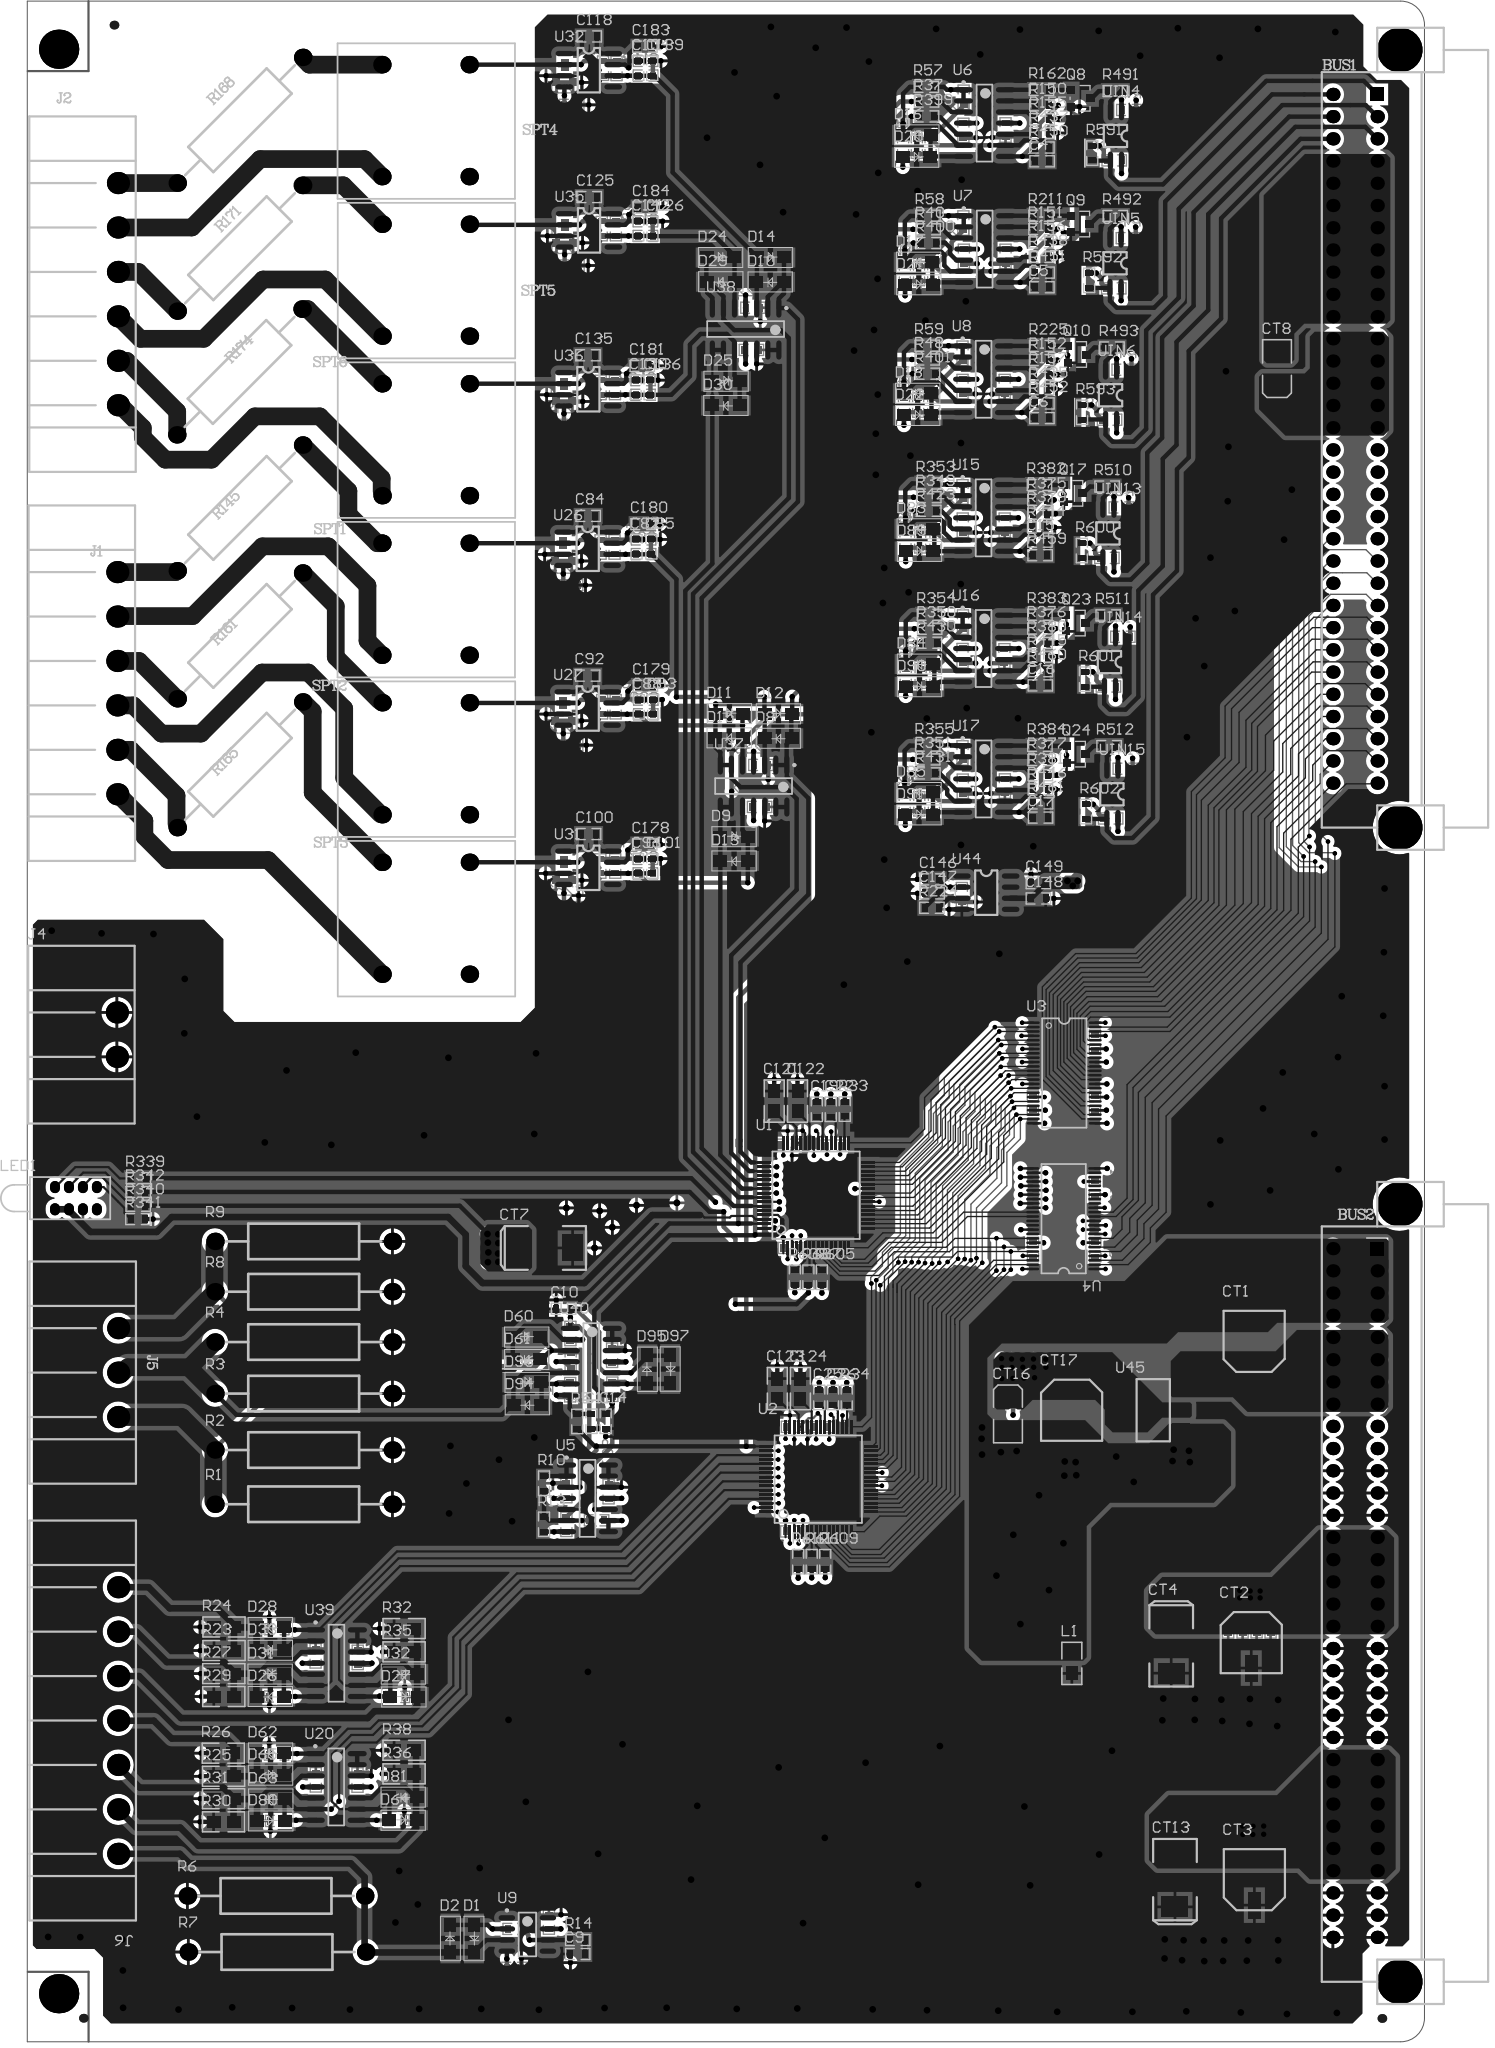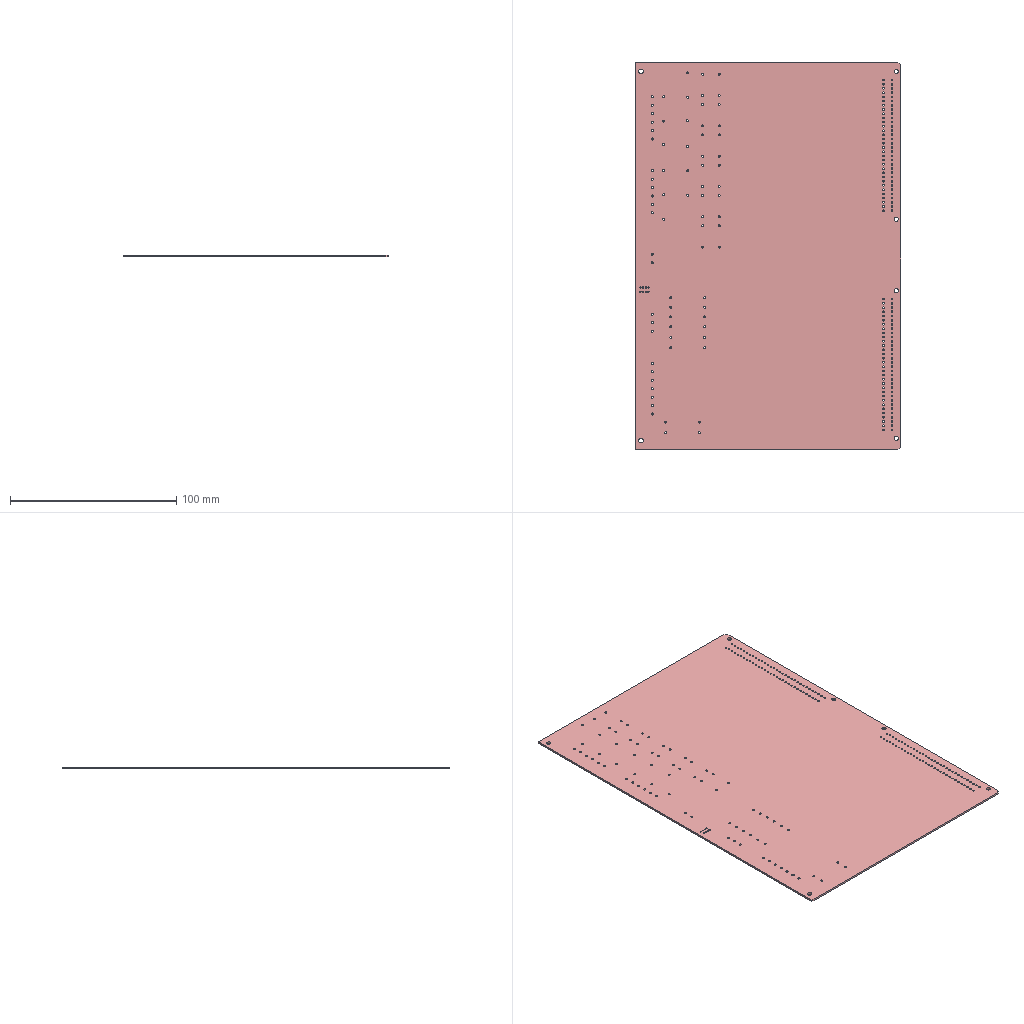Circuit board layout | Altium Designer | box 160 x 233.3 x 1.1 mm
Layer stack:
# Altium Designer layer stack of  (unit mm; dielectric type: 0 none, 1 core, 2 prepreg, 3 surface material)
index,name,kind,layer,copper_thickness_mm,dielectric_type,dielectric_thickness_mm,dielectric_material,dielectric_constant
0,TopPaste,other,,,,,,
1,TopOverlay,other,,,,,,
2,TopSolder,dielectric,,,3,0.0102,Solder Resist,3.5
3,TopLayer,copper,TopLayer,0.0356,,,,
4,Dielectric1,dielectric,,,1,0.32,FR-4,4.8
5,GND,copper,GND,0.0356,,,,
6,Dielectric2,dielectric,,,2,0.32,FR-4,4.8
7,POWER,copper,POWER,0.0356,,,,
8,Dielectric3,dielectric,,,1,0.32,FR-4,4.8
9,BottomLayer,copper,BottomLayer,0.0356,,,,
10,BottomSolder,dielectric,,,3,0.0102,Solder Resist,3.5
11,BottomOverlay,other,,,,,,
12,BottomPaste,other,,,,,,
# drill layer pairs: low layer,high layer
drill_pair,TopLayer,BottomLayer
Part placement:
Designator,Comment,Layer,Footprint,Center-X(mm),Center-Y(mm),Rotation
C253,0.1uF,BottomLayer,0603,62.306,129.743,180
C252,0.1uF,BottomLayer,0603,62.23,166.548,360
C251,0.1uF,BottomLayer,0603,62.382,203.098,180
C224,0.1uF,BottomLayer,0603,83.109,198.272,360
C194,0.1uF,BottomLayer,0603,37.846,43.967,270
R28,0,BottomLayer,0603,61.747,59.182,270
R12,10k_1%,BottomLayer,0603,65.202,59.639,360
C1,0.1uF,BottomLayer,0603,115.189,90.602,90
C2,0.1uF,BottomLayer,0603,122.326,90.602,270
C7,0.1uF,BottomLayer,0603,122.276,107.315,90
C8,0.1uF,BottomLayer,0603,115.164,107.34,270
R11,4.7k,BottomLayer,0603,55.88,12.929,180
C12,30p,BottomLayer,0603,28.575,47.193,360
C13,30p,BottomLayer,0603,28.55,32.868,360
C20,30p,BottomLayer,0603,28.575,39.497,360
C21,30p,BottomLayer,0603,28.677,25.273,360
C23,30p,BottomLayer,0603,42.393,39.446,180
C27,30p,BottomLayer,0603,42.342,25.349,180
C3,0.1uF,BottomLayer,0603,112.903,73.863,270
C18,1uF,BottomLayer,0603,92.329,102.489,360
C24,1uF,BottomLayer,0603,87.757,70.333,360
C83,1000p,BottomLayer,0603,70.587,170.104,360
C89,1000p,BottomLayer,0603,70.841,151.79,360
C97,1000p,BottomLayer,0603,70.79,133.604,360
C113,1000p,BottomLayer,0603,70.815,224.815,360
C119,0.1uF,BottomLayer,0603,87.046,102.591,360
C120,0.1uF,BottomLayer,0603,90.907,70.282,180
C128,0.1uF,BottomLayer,0603,87.427,90.78,360
C129,0.1uF,BottomLayer,0603,87.681,58.369,360
C132,1000p,BottomLayer,0603,70.536,188.316,360
C143,1000p,BottomLayer,0603,70.79,206.477,360
C156,0.1uF,BottomLayer,0603,124.485,215.113,360
C157,0.1uF,BottomLayer,0603,124.435,200.482,180
C158,0.1uF,BottomLayer,0603,123.952,185.471,180
C159,0.1uF,BottomLayer,0603,123.647,169.672,360
C163,0.1uF,BottomLayer,0603,123.825,154.965,180
C164,0.1uF,BottomLayer,0603,124.079,139.878,180
C165,0.1uF,BottomLayer,0603,122.276,114.3,270
C171,0.1uF,BottomLayer,0603,122.25,97.561,90
C173,0.1uF,BottomLayer,0603,137.541,47.574,90
C174,0.1uF,BottomLayer,0603,139.192,47.574,270
C175,0.1uF,BottomLayer,0603,140.792,47.6,270
C176,0.1uF,BottomLayer,0603,142.392,47.574,90
C177,0.1uF,BottomLayer,0603,61.747,63.043,90
C182,0.1uF,BottomLayer,0603,55.855,89.179,180
C192,0.1uF,BottomLayer,0603,37.821,29.947,270
C193,0.1uF,BottomLayer,0603,112.039,204.14,270
C195,0.1uF,BottomLayer,0603,55.753,8.484,360
C196,0.1uF,BottomLayer,0603,66.573,62.916,90
C197,0.1uF,BottomLayer,0603,66.98,78.511,270
C204,0.1uF,BottomLayer,0603,142.215,21.615,90
C205,0.1uF,BottomLayer,0603,140.589,21.59,90
C206,0.1uF,BottomLayer,0603,138.963,21.59,270
C215,0.1uF,BottomLayer,0603,107.213,218.542,270
C216,0.1uF,BottomLayer,0603,107.036,131.166,90
C217,0.1uF,BottomLayer,0603,107.112,158.496,90
C218,0.1uF,BottomLayer,0603,107.137,173.406,270
C219,0.1uF,BottomLayer,0603,107.264,204.14,90
C220,0.1uF,BottomLayer,0603,59.741,13.716,270
C230,0.1uF,BottomLayer,0603,33.045,29.972,270
C231,0.1uF,BottomLayer,0603,107.137,143.561,270
C232,0.1uF,BottomLayer,0603,107.112,189.255,270
C233,0.1uF,BottomLayer,0603,84.023,145.999,180
C234,0.1uF,BottomLayer,0603,62.23,77.927,90
C235,0.1uF,BottomLayer,0603,33.02,44.145,270
C238,0.1uF,BottomLayer,0603,111.912,158.471,90
C239,0.1uF,BottomLayer,0603,111.938,189.255,270
C240,0.1uF,BottomLayer,0603,82.931,193.446,360
C249,0.1uF,BottomLayer,0603,62.306,184.887,360
C254,0.1uF,BottomLayer,0603,62.23,148.26,360
C255,0.1uF,BottomLayer,0603,111.963,143.586,270
C256,0.1uF,BottomLayer,0603,111.938,173.406,90
C257,0.1uF,BottomLayer,0603,112.039,218.592,90
C261,0.1uF,BottomLayer,0603,62.357,221.463,180
C262,0.1uF,BottomLayer,0603,83.871,141.199,360
D42,BAV99W,BottomLayer,SOT23R,61.404,170.332,180
D44,BAV99W,BottomLayer,SOT23R,61.404,152.07,180
D46,BAV99W,BottomLayer,SOT23R,61.481,133.833,180
D48,BAV99W,BottomLayer,SOT23R,61.557,225.044,180
D51,BAV99W,BottomLayer,SOT23R,61.557,206.705,180
D53,BAV99W,BottomLayer,SOT23R,61.481,188.57,180
R67,10k,BottomLayer,0603,100.305,216.738,90
R70,10k,BottomLayer,0603,100.508,202.184,90
R71,10k,BottomLayer,0603,100.406,187.147,90
R76,10k,BottomLayer,0603,107.239,222.326,90
R85,4.7k,BottomLayer,0603,67.005,74.625,90
R86,10k,BottomLayer,0603,107.213,207.95,90
R87,10k,BottomLayer,0603,107.112,193.065,90
R93,4.7k,BottomLayer,0603,62.179,74.574,90
R97,4.7k,BottomLayer,0603,62.205,81.001,270
R100,10k,BottomLayer,0603,103.454,216.738,270
R105,5.1k_1%,BottomLayer,0603,65.659,189.154,90
R106,5.1k_1%,BottomLayer,0603,67.31,189.154,90
R108,10k,BottomLayer,0603,103.759,202.209,270
R110,5.1k_1%,BottomLayer,0603,67.412,207.315,90
R111,5.1k_1%,BottomLayer,0603,65.786,207.315,90
R113,5.1k,BottomLayer,0603,70.79,208.153,180
R117,10k,BottomLayer,0603,103.759,187.147,270
R118,5.1k,BottomLayer,0603,70.815,226.492,180
R119,5.1k_1%,BottomLayer,0603,67.488,225.628,90
R120,5.1k_1%,BottomLayer,0603,65.938,225.654,90
R124,5.1k,BottomLayer,0603,70.79,135.255,180
R125,5.1k_1%,BottomLayer,0603,67.335,134.442,90
R126,5.1k_1%,BottomLayer,0603,65.634,134.442,90
R130,5.1k,BottomLayer,0603,70.841,153.467,180
R131,5.1k_1%,BottomLayer,0603,65.837,152.654,90
R132,10k,BottomLayer,0603,101.879,216.738,270
R133,5.1k_1%,BottomLayer,0603,67.386,152.654,90
R137,5.1k,BottomLayer,0603,70.587,171.78,180
R138,5.1k_1%,BottomLayer,0603,65.659,170.917,90
R139,5.1k_1%,BottomLayer,0603,67.259,170.917,90
R146,10k,BottomLayer,0603,102.133,202.184,270
R147,10k,BottomLayer,0603,102.032,187.147,270
R357,10k,BottomLayer,0603,100.584,171.679,90
R358,10k,BottomLayer,0603,100.609,156.185,90
R359,10k,BottomLayer,0603,100.482,141.554,90
R360,10k,BottomLayer,0603,107.112,177.216,90
R361,10k,BottomLayer,0603,107.163,162.331,90
R362,10k,BottomLayer,0603,107.112,147.371,90
R364,10k,BottomLayer,0603,102.26,171.628,270
R365,10k,BottomLayer,0603,102.311,156.159,270
R366,10k,BottomLayer,0603,103.835,141.554,270
R372,10k,BottomLayer,0603,104.013,171.628,270
R373,10k,BottomLayer,0603,104.013,156.185,270
R374,10k,BottomLayer,0603,102.159,141.554,270
R414,5.1k,BottomLayer,0603,70.536,189.992,180
R486,2k,BottomLayer,0603,126.162,220.878,180
R487,2k,BottomLayer,0603,126.111,206.223,180
R488,2k,BottomLayer,0603,125.628,191.186,180
R503,2k,BottomLayer,0603,125.298,175.438,180
R506,2k,BottomLayer,0603,125.476,160.655,180
R507,2k,BottomLayer,0603,125.755,145.567,180
R342,3.3k,TopLayer,0603,12.7,97.18,360
R38,2k,TopLayer,0805,43.155,33.35,180
R36,2k,TopLayer,0805,43.155,30.658,180
R35,2k,TopLayer,0805,43.155,44.602,180
R32,2k,TopLayer,0805,43.155,47.269,180
R31,2k,TopLayer,0805,22.479,27.813,180
R30,2k,TopLayer,0805,22.479,25.171,180
R29,2k,TopLayer,0805,22.504,39.497,180
R27,2k,TopLayer,0805,22.504,42.113,180
R26,2k,TopLayer,0805,22.454,33.02,180
R25,2k,TopLayer,0805,22.479,30.378,180
R24,2k,TopLayer,0805,22.53,47.447,180
R23,2k,TopLayer,0805,22.53,44.755,180
U5,TL064I,TopLayer,TL064D_SOIC-14,64.16,62.154,0
R13,10k_1%,TopLayer,0603,59.182,59.182,90
R10,10k_1%,TopLayer,0603,59.182,63.881,90
R5,0,TopLayer,0603,62.992,70.942,90
J5,Header3,TopLayer,EDGCON_3p_5.08mm_ear,10.414,76.53,270
SPT6,SPT204A,TopLayer,SPT204A,45.64,183.184,360
SPT5,SPT204A,TopLayer,SPT204A,45.64,201.421,360
SPT4,SPT204A,TopLayer,SPT204A,45.615,219.658,360
SPT3,SPT204A,TopLayer,SPT204A,45.64,128.472,360
SPT2,SPT204A,TopLayer,SPT204A,45.64,146.71,360
SPT1,SPT204A,TopLayer,SPT204A,45.615,164.947,360
R174,50kO_2W_1%,TopLayer,AXIAL0.8,24.309,190.925,225
R171,50kO_2W_1%,TopLayer,AXIAL0.8,24.36,205.073,225
R168,50kO_2W_1%,TopLayer,AXIAL0.8,24.36,219.703,225
R165,50kO_2W_1%,TopLayer,AXIAL0.8,24.36,146.018,225
R161,50kO_2W_1%,TopLayer,AXIAL0.8,24.36,160.75,225
R145,50kO_2W_1%,TopLayer,AXIAL0.8,24.36,175.38,225
BUS2,CON64,TopLayer,BUS64W-A,153.34,51.333,270
BUS1,CON64,TopLayer,BUS64W-A,153.34,183.286,270
J1,CON6,TopLayer,EDGCon_6P_5.08mm_ear,10.312,155.346,270
J2,CON6,TopLayer,EDGCon_6P_5.08mm_ear,10.389,199.822,270
U3,SN74LVCH16T245_TSSOP48,TopLayer,SN74LVC16245_TSSOP48,118.764,110.779,0
U4,SN74LVCH16T245_TSSOP48,TopLayer,SN74LVC16245_TSSOP48,118.7,94.123,180
D1,1N4148,TopLayer,1N4148-A,51.156,11.836,270
D2,1N4148,TopLayer,1N4148-A,48.463,11.836,90
R6,2W_1%,TopLayer,AXIAL0.8,28.49,16.701,360
R7,2W_1%,TopLayer,AXIAL0.8,28.6,10.287,360
U9,TL061D,TopLayer,TL061_SOIC8,57.277,12.294,0
C9,0.1uF,TopLayer,0603,63.043,10.058,0
R14,10k,TopLayer,0603,63.043,11.659,180
LED1,LEDGroup_4,TopLayer,LEDGroup_4,5.575,96.469,360
J4,Header2,TopLayer,EDGCON_2p_5.08mm_ear,10.262,115.164,270
J6,Header7,TopLayer,EDGCon_7P_5.08mm_ear,10.414,36.754,270
C10,30p,TopLayer,0603,61.417,83.82,360
C11,30p,TopLayer,0603,64.618,70.968,90
C14,30p,TopLayer,0603,66.243,70.968,90
C4,0.1uF,TopLayer,0603,116.23,215.011,360
C5,0.1uF,TopLayer,0603,116.205,200.609,360
C6,0.1uF,TopLayer,0603,116.205,185.649,0
C15,0.1uF,TopLayer,0603,115.976,171.526,360
C16,0.1uF,TopLayer,0603,116.027,155.092,360
C17,0.1uF,TopLayer,0603,116.053,139.979,360
C19,1uF,TopLayer,0603,90.424,106.629,270
C22,1uF,TopLayer,0603,92.024,106.629,270
C25,1uF,TopLayer,0603,90.703,73.685,270
C26,1uF,TopLayer,0603,92.278,73.685,270
C82,680p,TopLayer,0603,69.774,170.942,90
C84,30p,TopLayer,0603,64.237,174.473,180
C85,30p,TopLayer,0603,71.476,170.942,270
C88,680p,TopLayer,0603,70.028,152.629,90
C92,30p,TopLayer,0603,64.186,156.21,180
C93,30p,TopLayer,0603,71.679,152.629,270
C96,680p,TopLayer,0603,69.952,134.442,90
C100,30p,TopLayer,0603,64.287,138.1,180
C101,30p,TopLayer,0603,71.577,134.442,270
C104,680p,TopLayer,0603,69.977,225.654,90
C118,30p,TopLayer,0603,64.364,229.286,180
C121,10u,TopLayer,0805,85.547,107.569,270
C122,10u,TopLayer,0805,88.214,107.569,270
C123,10u,TopLayer,0805,85.903,74.701,270
C124,10u,TopLayer,0805,88.544,74.701,270
C125,30p,TopLayer,0603,64.364,210.922,180
C126,30p,TopLayer,0603,71.603,207.315,270
C130,680p,TopLayer,0603,69.672,189.179,90
C135,30p,TopLayer,0603,64.211,192.837,180
C136,30p,TopLayer,0603,71.272,189.154,270
C139,30p,TopLayer,0603,71.577,225.654,270
C142,680p,TopLayer,0603,69.977,207.315,90
C146,1uF,TopLayer,0603,103.632,132.918,180
C147,0.1uF,TopLayer,0603,103.632,131.318,180
C148,1uF,TopLayer,0603,115.799,130.734,360
C149,0.1uF,TopLayer,0603,115.799,132.486,360
C178,0.1uF,TopLayer,0603,70.714,136.906,180
C179,0.1uF,TopLayer,0603,70.79,155.042,180
C180,0.1uF,TopLayer,0603,70.536,173.533,360
C181,0.1uF,TopLayer,0603,70.434,191.618,360
C183,0.1uF,TopLayer,0603,70.739,228.117,180
C184,0.1uF,TopLayer,0603,70.764,209.728,360
CT1,100uF/16V,TopLayer,L470UF,140.513,80.099,180
CT2,100uF/35V,TopLayer,L470UF,140.183,45.657,0
CT3,100uF/35V,TopLayer,L470UF,140.538,18.555,180
CT8,22u/16V,TopLayer,3528_CASE-B,143.129,191.376,90
CT17,100uF/16V,TopLayer,L470UF,119.609,72.225,360
D8,1N4148,TopLayer,1N4148-A,86.03,149.047,180
D9,1N4148,TopLayer,1N4148-A,80.95,137.795,360
D10,1N4148,TopLayer,1N4148-A,85.09,201.219,180
D11,1N4148,TopLayer,1N4148-A,80.416,151.867,360
D12,1N4148,TopLayer,1N4148-A,86.03,151.841,360
D13,1N4148,TopLayer,1N4148-A,80.95,135.026,180
D14,1N4148,TopLayer,1N4148-A,85.115,204.013,360
D15,1N4148,TopLayer,1N4148-A,80.391,149.098,180
D16,1N4148,TopLayer,1N4148-A,101.879,218.034,180
D17,1N4148,TopLayer,1N4148-A,102.083,203.479,180
D18,1N4148,TopLayer,1N4148-A,101.981,188.493,180
D20,1N4148,TopLayer,1N4148-A,101.854,215.468,360
D21,1N4148,TopLayer,1N4148-A,102.108,200.889,360
D22,1N4148,TopLayer,1N4148-A,101.981,185.953,360
D24,1N4148,TopLayer,1N4148-A,79.4,204.013,360
D25,1N4148,TopLayer,1N4148-A,80.035,189.865,360
D26,1N4148,TopLayer,1N4148-A,27.838,39.497,180
D27,1N4148,TopLayer,1N4148-A,43.129,39.446,360
D28,1N4148,TopLayer,1N4148-A,27.838,47.396,180
D29,1N4148,TopLayer,1N4148-A,79.426,201.244,180
D30,1N4148,TopLayer,1N4148-A,80.01,187.096,180
D31,1N4148,TopLayer,1N4148-A,27.813,42.062,360
D32,1N4148,TopLayer,1N4148-A,43.078,42.062,180
D33,1N4148,TopLayer,1N4148-A,27.838,44.78,360
D60,1N4148,TopLayer,1N4148-A,57.201,80.594,360
D61,1N4148,TopLayer,1N4148-A,57.201,78.029,180
D62,1N4148,TopLayer,1N4148-A,27.864,33.045,180
D63,1N4148,TopLayer,1N4148-A,27.889,27.788,180
D64,1N4148,TopLayer,1N4148-A,43.053,25.349,360
D65,1N4148,TopLayer,1N4148-A,27.864,30.505,360
D80,1N4148,TopLayer,1N4148-A,27.889,25.273,360
D81,1N4148,TopLayer,1N4148-A,43.053,27.991,180
D83,1N4148,TopLayer,1N4148-A,102.159,172.999,180
D84,1N4148,TopLayer,1N4148-A,102.184,157.531,180
D85,1N4148,TopLayer,1N4148-A,102.133,142.85,180
D89,1N4148,TopLayer,1N4148-A,102.184,170.409,360
D90,1N4148,TopLayer,1N4148-A,102.184,154.94,360
D91,1N4148,TopLayer,1N4148-A,102.133,140.284,360
D94,1N4148,TopLayer,1N4148-A,57.277,72.847,180
D95,1N4148,TopLayer,1N4148-A,71.018,76.911,90
D96,1N4148,TopLayer,1N4148-A,57.252,75.413,360
D97,1N4148,TopLayer,1N4148-A,73.635,76.937,270
L1,1uH,TopLayer,0805,119.634,43.282,270
Q8,2N2222,TopLayer,SOT23-3,120.637,222.212,270
Q9,2N2222,TopLayer,SOT23-3,120.587,207.835,270
Q10,2N2222,TopLayer,SOT23-3,120.231,192.926,270
Q17,2N2222,TopLayer,SOT23-3,119.799,177.051,270
Q23,2N2222,TopLayer,SOT23-3,120.079,162.217,270
Q24,2N2222,TopLayer,SOT23-3,120.104,147.231,270
R1,100O_2W_1%,TopLayer,AXIAL0.8,31.657,61.48,180
R2,100O_2W_1%,TopLayer,AXIAL0.8,31.657,67.678,180
R3,100O_2W_1%,TopLayer,AXIAL0.8,31.657,74.129,180
R4,100O_2W_1%,TopLayer,AXIAL0.8,31.657,80.022,180
R8,100O_2W_1%,TopLayer,AXIAL0.8,31.657,85.776,180
R9,100O_2W_1%,TopLayer,AXIAL0.8,31.657,91.528,180
R33,10k,TopLayer,0603,93.624,106.655,90
R34,10k,TopLayer,0603,93.853,73.685,90
R37,10k,TopLayer,0603,102.997,221.844,180
R40,10k,TopLayer,0603,103.175,207.239,180
R48,10k,TopLayer,0603,103.073,192.354,180
R57,10k,TopLayer,0603,102.972,223.52,360
R58,10k,TopLayer,0603,103.149,208.788,360
R59,10k,TopLayer,0603,103.073,193.929,360
R150,10k,TopLayer,0603,116.205,221.412,360
R151,10k,TopLayer,0603,116.103,207.264,360
R152,10k,TopLayer,0603,116.18,192.278,360
R155,10k,TopLayer,0603,116.23,219.837,360
R156,10k,TopLayer,0603,116.103,205.74,360
R157,10k,TopLayer,0603,116.18,190.627,360
R162,10k,TopLayer,0603,116.154,223.164,180
R211,10k,TopLayer,0603,116.103,208.788,180
R224,0,TopLayer,0603,103.607,129.667,180
R225,10k,TopLayer,0603,116.18,193.904,180
R339,3.3k,TopLayer,0603,12.725,98.755,360
R340,10k,TopLayer,0603,12.7,95.606,360
R341,10k,TopLayer,0603,12.675,94.082,360
R349,10k,TopLayer,0603,103.251,176.606,180
R350,10k,TopLayer,0603,103.353,161.569,180
R351,10k,TopLayer,0603,103.124,146.634,180
R353,10k,TopLayer,0603,103.251,178.181,360
R354,10k,TopLayer,0603,103.327,163.17,360
R355,10k,TopLayer,0603,103.124,148.209,360
R375,10k,TopLayer,0603,115.976,176.301,360
R376,10k,TopLayer,0603,115.976,161.595,360
R377,10k,TopLayer,0603,116.002,146.558,360
R379,10k,TopLayer,0603,115.976,174.727,360
R380,10k,TopLayer,0603,116.002,159.944,360
R381,10k,TopLayer,0603,116.027,144.831,360
R382,10k,TopLayer,0603,115.926,178.003,180
R383,10k,TopLayer,0603,115.976,163.17,180
R384,10k,TopLayer,0603,115.976,148.184,180
R399,5.1k,TopLayer,0603,102.997,220.142,180
R400,5.1k,TopLayer,0603,103.2,205.664,180
R401,5.1k,TopLayer,0603,103.099,190.729,180
R423,5.1k,TopLayer,0603,103.251,175.057,180
R430,5.1k,TopLayer,0603,103.327,159.969,180
R431,5.1k,TopLayer,0603,103.149,145.034,180
R435,2.4k,TopLayer,0603,116.18,188.951,360
R437,2.4k,TopLayer,0603,116.205,218.237,360
R438,2.4k,TopLayer,0603,116.154,204.089,360
R444,2.4k,TopLayer,0603,115.951,173.152,360
R445,2.4k,TopLayer,0603,116.027,158.369,360
R446,2.4k,TopLayer,0603,116.027,143.205,360
R450,5.6k,TopLayer,0603,116.205,216.586,360
R451,5.6k,TopLayer,0603,116.23,202.286,360
R452,5.6k,TopLayer,0603,116.205,187.325,360
R459,5.6k,TopLayer,0603,116.002,169.977,360
R460,5.6k,TopLayer,0603,116.027,156.718,360
R461,5.6k,TopLayer,0603,116.053,141.605,360
R491,2k,TopLayer,0603,124.612,223.037,180
R492,2k,TopLayer,0603,124.612,208.763,180
R493,2k,TopLayer,0603,124.231,193.726,180
R510,2k,TopLayer,0603,123.673,177.825,180
R511,2k,TopLayer,0603,123.8,163.093,180
R512,2k,TopLayer,0603,123.901,148.158,180
R591,10k,TopLayer,0603,121.971,215.951,270
R592,10k,TopLayer,0603,121.615,201.397,270
R593,10k,TopLayer,0603,120.802,186.309,270
R600,10k,TopLayer,0603,120.777,170.51,270
R601,10k,TopLayer,0603,121.133,155.804,270
R602,10k,TopLayer,0603,121.26,140.665,270
R605,4.7k,TopLayer,0603,91.008,87.427,270
R607,4.7k,TopLayer,0603,89.459,87.427,270
R608,4.7k,TopLayer,0603,87.909,87.427,270
R609,4.7k,TopLayer,0603,91.389,54.915,270
R611,4.7k,TopLayer,0603,89.84,54.915,270
R612,4.7k,TopLayer,0603,88.29,54.915,270
U26,OP07CS,TopLayer,SO-8,64.186,170.713,0
U27,OP07CS,TopLayer,SO-8,64.186,152.451,0
U31,OP07CS,TopLayer,SO-8,64.262,134.239,0
U32,OP07CS,TopLayer,SO-8,64.313,225.425,0
U35,OP07CS,TopLayer,SO-8,64.338,207.112,0
U36,OP07CS,TopLayer,SO-8,64.262,188.951,0
U44,REF195,TopLayer,SO-8,109.83,131.394,360
U45,AS1117-3.3V,TopLayer,SOT223,128.956,72.225,90
CT4,22u/35V,TopLayer,7343_CASE-D,131.013,45.288,90
CT7,22u/35V,TopLayer,7343_CASE-D,59.334,90.78,180
CT13,22u/35V,TopLayer,7343_CASE-D,131.445,18.567,270
CT16,22u/16V,TopLayer,3528_CASE-B,112.319,71.742,270
U1,AD7606,TopLayer,AD7606_LQFP64,90.339,96.805,90
U2,AD7606,TopLayer,AD7606_LQFP64,90.593,64.344,90
U6,TL064I,TopLayer,TL064D_SOIC-14,109.626,219.38,0
U7,TL064I,TopLayer,TL064D_SOIC-14,109.652,204.978,0
U8,TL064I,TopLayer,TL064D_SOIC-14,109.525,190.094,0
U15,TL064I,TopLayer,TL064D_SOIC-14,109.525,174.244,0
U16,TL064I,TopLayer,TL064D_SOIC-14,109.525,159.309,0
U17,TL064I,TopLayer,TL064D_SOIC-14,109.525,144.399,0
U20,TL064I,TopLayer,TL064D_SOIC-14,35.382,29.159,0
U37,TL064I,TopLayer,TL064D_SOIC-14,83.185,143.586,270
U38,TL064I,TopLayer,TL064D_SOIC-14,82.271,195.834,270
U39,TL064I,TopLayer,TL064D_SOIC-14,35.408,43.307,0
U40,TL064I,TopLayer,TL064D_SOIC-14,64.592,77.775,360
UIN4,TLP285,TopLayer,TLP285_SOP4,124.689,217.907,270
UIN5,TLP285,TopLayer,TLP285_SOP4,124.638,203.352,270
UIN6,TLP285,TopLayer,TLP285_SOP4,124.13,188.265,270
UIN13,TLP285,TopLayer,TLP285_SOP4,123.825,172.466,270
UIN14,TLP285,TopLayer,TLP285_SOP4,124.003,157.759,270
UIN15,TLP285,TopLayer,TLP285_SOP4,124.282,142.646,270
Pad and via stacks:
# Altium Designer via and pad stacks of  (unit mm). Each distinct definition once, with the count of objects using it.
# via: kind,start_layer,end_layer,hole_mm,diameter_mm,mode(0 simple;1 top-mid-bottom;2 full stack),diameter_per_layer,count,example_net
# pad: kind,layer,hole_mm,hole_type(0 round;1 square;2 slot),plating,top_size,top_shape(1 round;2 rect;3 octagon;9 rounded rect),mid_size,bottom_size,mode,footprint,size_per_layer,count,example
pad,TopLayer,0,0,plated,1x1,1,1x1,1x1,0,,,3,0
pad,TopLayer,0,0,plated,0.635x0.8128,2,0.635x0.8128,0.635x0.8128,0,0603,,238,C88.2
pad,TopLayer,0,0,plated,1.524x1.27,2,1.524x1.27,1.524x1.27,0,0805,,34,R26.1
pad,TopLayer,0,0,plated,1.5x0.3,1,1.5x0.3,1.5x0.3,0,SN74LVC16245_TSSOP48,,96,U3.1
pad,TopLayer,0,0,plated,1.524x1.27,2,1.524x1.27,1.524x1.27,0,1N4148-A,,88,D2.A
pad,TopLayer,0,0,plated,0.6x1.9,1,0.6x1.9,0.6x1.9,0,TL061_SOIC8,,8,U9.1
pad,TopLayer,0,0,plated,2.032x0.6096,1,2.032x0.6096,2.032x0.6096,0,SO-8,,56,U36.8
pad,TopLayer,0,0,plated,3.048x1.397,2,3.048x1.397,3.048x1.397,0,L470UF,,8,CT1.2
pad,TopLayer,0,0,plated,1.499x2.007,2,1.499x2.007,1.499x2.007,0,SOT223,,3,U45.2
pad,TopLayer,0,0,plated,3.81x2.007,2,3.81x2.007,3.81x2.007,0,SOT223,,1,U45.2
pad,TopLayer,0,0,plated,0.9144x1.016,2,0.9144x1.016,0.9144x1.016,0,SOT23-3,,6,Q24.C
pad,TopLayer,0,0,plated,0.9144x0.9144,2,0.9144x0.9144,0.9144x0.9144,0,SOT23-3,,12,Q24.E
pad,TopLayer,0,0,plated,1.905x2.286,2,1.905x2.286,1.905x2.286,0,3528_CASE-B,,4,CT8.1
pad,TopLayer,0,0,plated,2.4x3,2,2.4x3,2.4x3,0,7343_CASE-D,,6,CT13.1
pad,TopLayer,0,0,plated,0.6x2.2,1,0.6x2.2,0.6x2.2,0,TL064D_SOIC-14,,168,U5.1
pad,TopLayer,0,0,plated,2.032x0.6096,1,2.032x0.6096,2.032x0.6096,0,TLP285_SOP4,,24,UIN15.1
pad,TopLayer,0,0,plated,0.254x1.524,2,0.254x1.524,0.254x1.524,0,AD7606_LQFP64,,126,U1.12
pad,TopLayer,0,0,plated,0.254x1.524,1,0.254x1.524,0.254x1.524,0,AD7606_LQFP64,,2,U1.1
pad,BottomLayer,0,0,plated,0.635x0.8128,2,0.635x0.8128,0.635x0.8128,0,0603,,252,C159.2
pad,BottomLayer,0,0,plated,1x1,1,1x1,1x1,0,,,3,0
pad,BottomLayer,0,0,plated,0.9144x1.27,2,0.9144x1.27,0.9144x1.27,0,SOT23R,,6,D53.3
pad,BottomLayer,0,0,plated,0.9144x0.9144,2,0.9144x0.9144,0.9144x0.9144,0,SOT23R,,12,D53.1
pad,MultiLayer,1.295,0,plated,2.54x2.54,1,2.54x2.54,2.54x2.54,0,EDGCon_6P_5.08mm_ear,,12,J2.5
pad,MultiLayer,1.295,0,plated,2.54x2.54,1,2.54x2.54,2.54x2.54,0,EDGCon_7P_5.08mm_ear,,7,J6.7
pad,MultiLayer,1.016,0,plated,1.524x1.524,1,1.524x1.524,1.524x1.524,0,BUS64W-A,,126,BUS2.A31
pad,MultiLayer,2.54,0,plated,5.08x5.08,1,5.08x5.08,5.08x5.08,0,BUS64W-A,,4,BUS2.0
pad,MultiLayer,1.016,0,plated,1.524x1.524,2,1.524x1.524,1.524x1.524,0,BUS64W-A,,2,BUS2.A1
pad,MultiLayer,1.2,0,plated,2x2,1,2x2,2x2,0,SPT204A,,24,SPT3.3
pad,MultiLayer,2.7,0,plated,4.5x4.5,1,4.5x4.5,4.5x4.5,0,,,2,1
pad,MultiLayer,0.8128,0,plated,1.397x1.143,1,1.397x1.143,1.397x1.143,0,LEDGroup_4,,8,LED1.2
pad,MultiLayer,1.295,0,plated,2.54x2.54,1,2.54x2.54,2.54x2.54,0,EDGCON_3p_5.08mm_ear,,3,J5.3
pad,MultiLayer,1.2,0,plated,2x2,1,2x2,2x2,0,AXIAL0.8,,28,R145.1
pad,MultiLayer,1.295,0,plated,2.54x2.54,1,2.54x2.54,2.54x2.54,0,EDGCON_2p_5.08mm_ear,,2,J4.2
via,TopLayer,BottomLayer,0.381,0.762,0,,197,AGND
via,TopLayer,BottomLayer,0.3048,0.6096,0,,342,ISA
via,TopLayer,BottomLayer,0.254,0.508,0,,101,GND
Copper pours:
name,layer,net,type(0 solid;1 hatched;2 none)
Top Layer-No Net,TopLayer,GND,0
Top Layer-No Net,TopLayer,AGND,0
Top Layer-No Net,TopLayer,GND,0
Top Layer-No Net,TopLayer,+15V,0
TopLayer-No Net,TopLayer,+5V,0
TopLayer-No Net,TopLayer,+5V,0
TopLayer-No Net,TopLayer,+3.3V,0
Top Layer-No Net,TopLayer,+5VREF,0
TopLayer-No Net,TopLayer,+15V,0
TopLayer-No Net,TopLayer,-15V,0
Top Layer-No Net,BottomLayer,AGND,0
Top Layer-No Net,BottomLayer,+5VREF,0
TopLayer-No Net,BottomLayer,+15V,0
TopLayer-No Net,BottomLayer,-15V,0
Design rules, without the lines most boards share:
# Altium Designer design rules of  (exported by Altium Designer, unit mm)
# columns: name | kind | enabled | priority | scope1 | scope2 | descriptor | typed fields (field=value)
PolygonConnect_1 | 20 | enabled | 1 | InNet(AGND) | All | Polygon Connect Rule(Relief Connect )(Conductor Width=0.305mm) (Relief Angle=90 Angle) (Entries=4) (Air Gap Width=0.254mm) (InNet(AGND)),(All) | connect_style(0=relief,1=direct,2=none)=0 relief_conductor_width=0.3048 relief_entries=4
Clearance_1 | 0 | enabled | 1 | inpolygon{AGND} | All | Clearance Constraint (Gap=0.508mm) (inpolygon{AGND}),(All) | gap=0.508
NetAntennae | 56 | enabled | 1 | All | All | Net Antennae (Tolerance=0mm) (All) |
SilkToSilkClearance | 55 | enabled | 1 | All | All | Silk to Silk (Clearance=0mm) (All),(All) |
SilkscreenOverComponentPads | 54 | enabled | 1 | IsPad | All | Silk To Solder Mask (Clearance=0mm) (IsPad),(All) |
MinimumSolderMaskSliver | 53 | enabled | 1 | All | All | Minimum Solder Mask Sliver (Gap=0mm) (All),(All) |
HoleToHoleClearance | 52 | enabled | 1 | All | All | Hole To Hole Clearance (Gap=0mm) (All),(All) | gap=0
HoleSize | 42 | enabled | 1 | All | All | Hole Size Constraint (Min=0.025mm) (Max=25.4mm) (All) |
ComponentClearance | 24 | enabled | 1 | All | All | Component Clearance Constraint ( Horizontal Gap = 0.254mm, Vertical Gap = 0.254mm ) (All),(All)  | gap=0.254
Testpoint | 43 | enabled | 1 | (IsPad And (OnTopLayer Or OnBottomLayer)) | All | Fabrication Testpoint Style (Under Component=Yes) ((IsPad And (OnTopLayer Or OnBottomLayer))) |
TestPointUsage | 44 | enabled | 1 | All | All | Fabrication Testpoint Usage (Valid =One Required, Allow multiple per net=No) (All) |
SolderMaskExpansion | 13 | enabled | 1 | All | All | Solder Mask Expansion (Expansion =0.102mm) (All) | expansion=0.1016
PasteMaskExpansion | 14 | enabled | 1 | All | All | Paste Mask Expansion (Expansion =0mm) (All) | expansion=0
RoutingVias | 11 | enabled | 1 | All | All | Routing Via (MinHoleWidth=0.254mm) (MaxHoleWidth=0.305mm) (PreferredHoleWidth=0.254mm) (MinWidth=0.508mm) (MaxWidth=0.61mm) (PreferedWidth=0.508mm) (All) | via_min_hole=0.254 via_max_hole=0.3048 via_preferred_diameter=0.508 via_preferred_hole=0.254
RoutingCorners | 10 | enabled | 1 | All | All | Routing Corners (Style=45-Degree) (Min Setback=2.54mm) (Max Setback=2.54mm) (All) |
Width | 2 | enabled | 1 | All | All | Width Constraint (Min=0.152mm) (Max=2.54mm) (Preferred=0.152mm) (All) |
PolygonConnect | 20 | enabled | 2 | All | All | Polygon Connect Rule(Direct Connect )(Conductor Width=0.254mm) (Relief Angle=90 Angle) (Entries=4) (Air Gap Width=0.254mm) (All),(All) | connect_style(0=relief,1=direct,2=none)=1 relief_conductor_width=0.254 relief_entries=4
PlaneClearance | 12 | enabled | 1 | All | All | Power Plane Clearance (Clearance =0.508mm) (All) | clearance=0.508
PlaneConnect | 6 | enabled | 1 | All | All | Power Plane Connect Rule(Direct Connect )(Expansion=0.508mm) (Conductor Width=0.254mm) (Air Gap=0.254mm) (Entries=4) (All) | relief_conductor_width=0.254 relief_entries=4 relief_expansion=0.508
Clearance | 0 | enabled | 2 | All | All | Clearance Constraint (Gap=0.14mm) (All),(All) | gap=0.1397
Height | 50 | enabled | 1 | All | All | Height Constraint (Min=0mm) (Max=25.4mm) (Prefered=12.7mm) (All) | min_height=0 max_height=25.4
DiffPairsRouting | 51 | enabled | 1 | All | All | Differential Pairs Uncoupled Length using the Gap Constraints (Min=0.254mm) (Max=0.254mm) (Prefered=0.254mm)  and Width Constraints (Min=0.381mm) (Max=0.381mm) (Prefered=0.381mm) (All) |
Classes set for this board:
# Altium Designer classes of  (member kind: 0 net, 1 component, 2 from-to, 3 pad, 4 layer, 5 differential pair, 6 design channel, 7 polygon, 8 structure, 9 xSignal)
# columns: class name | member kind | superclass | members
All From-Tos | 0 | yes |